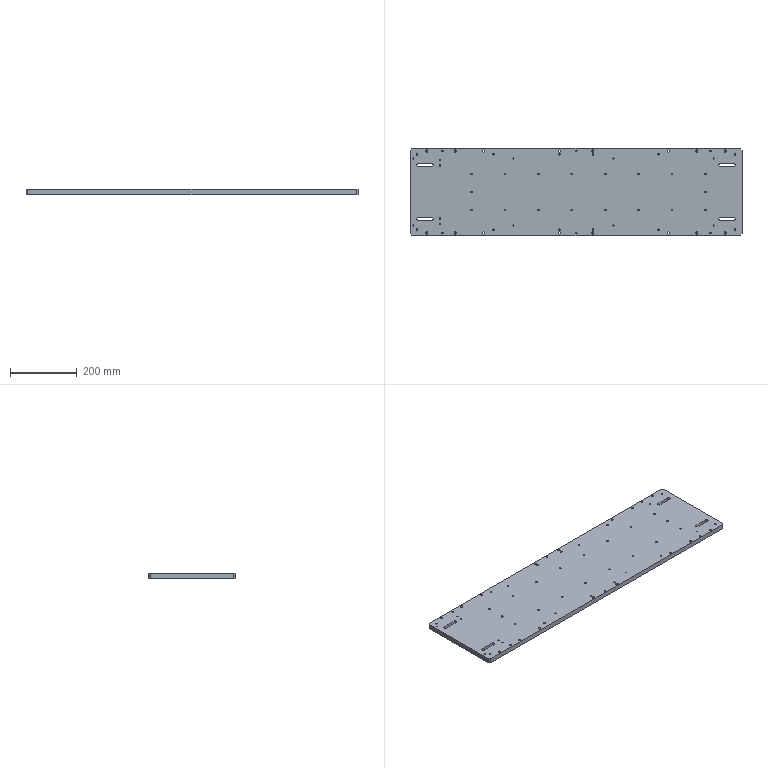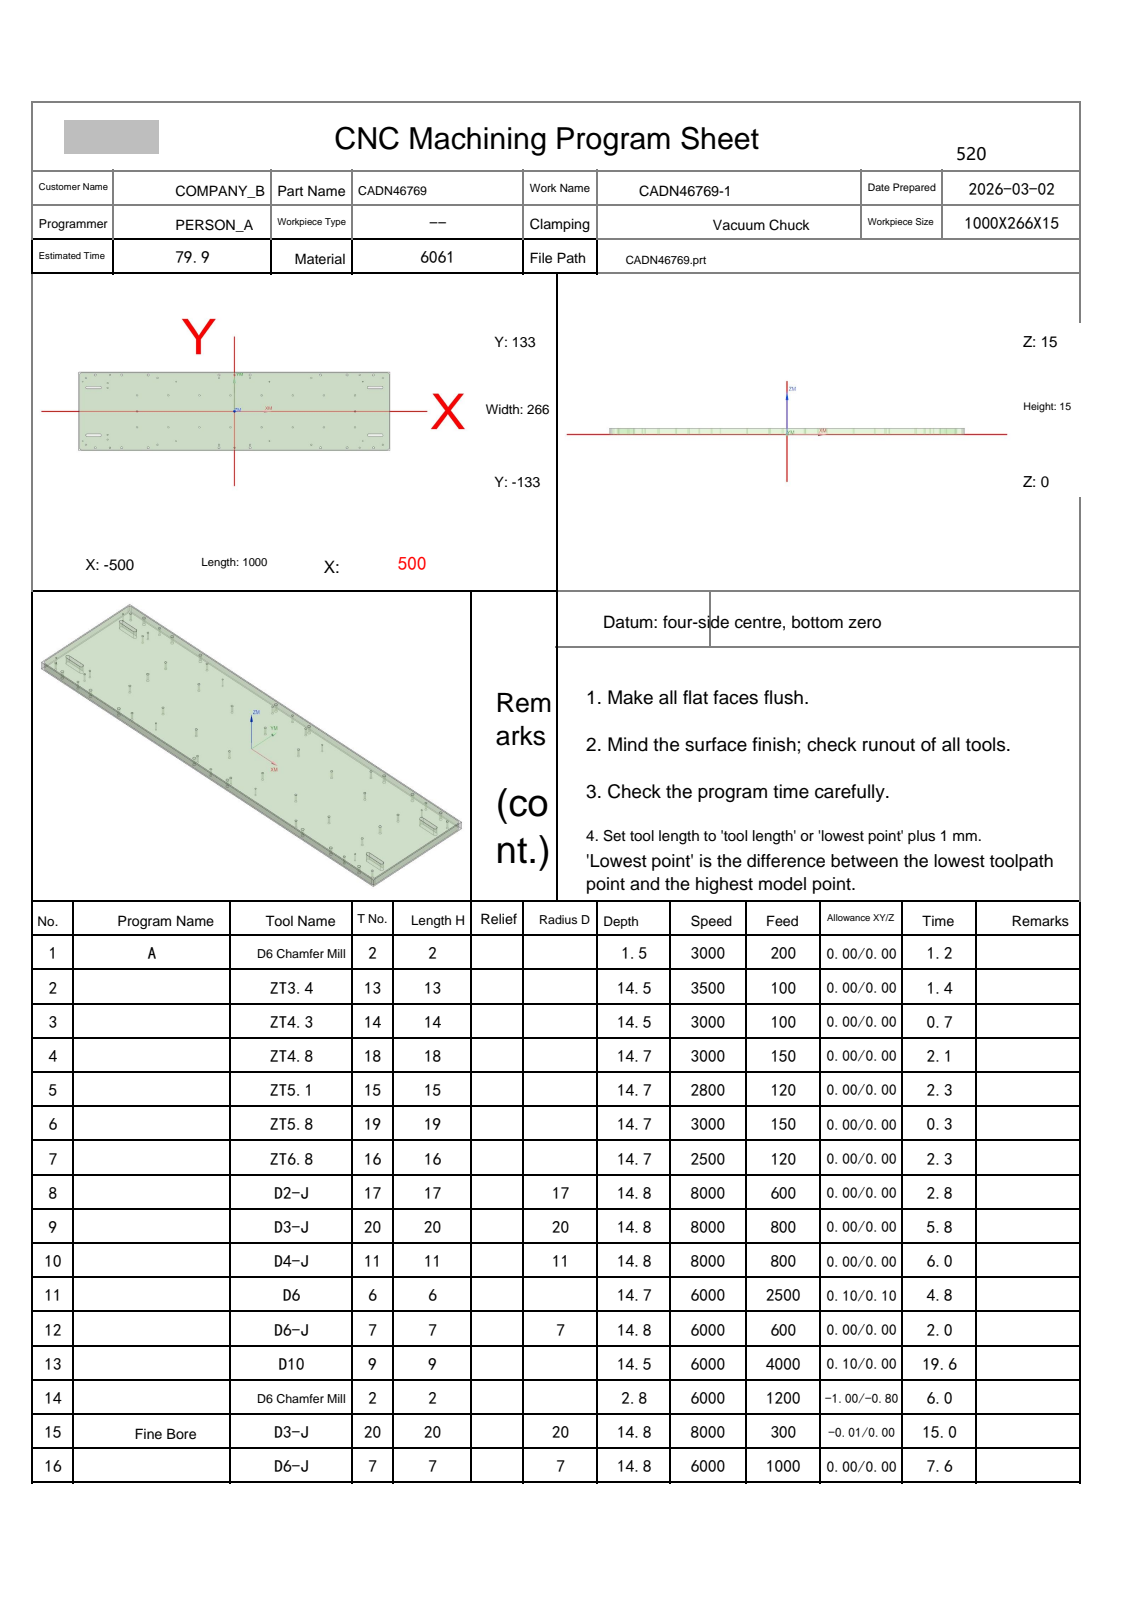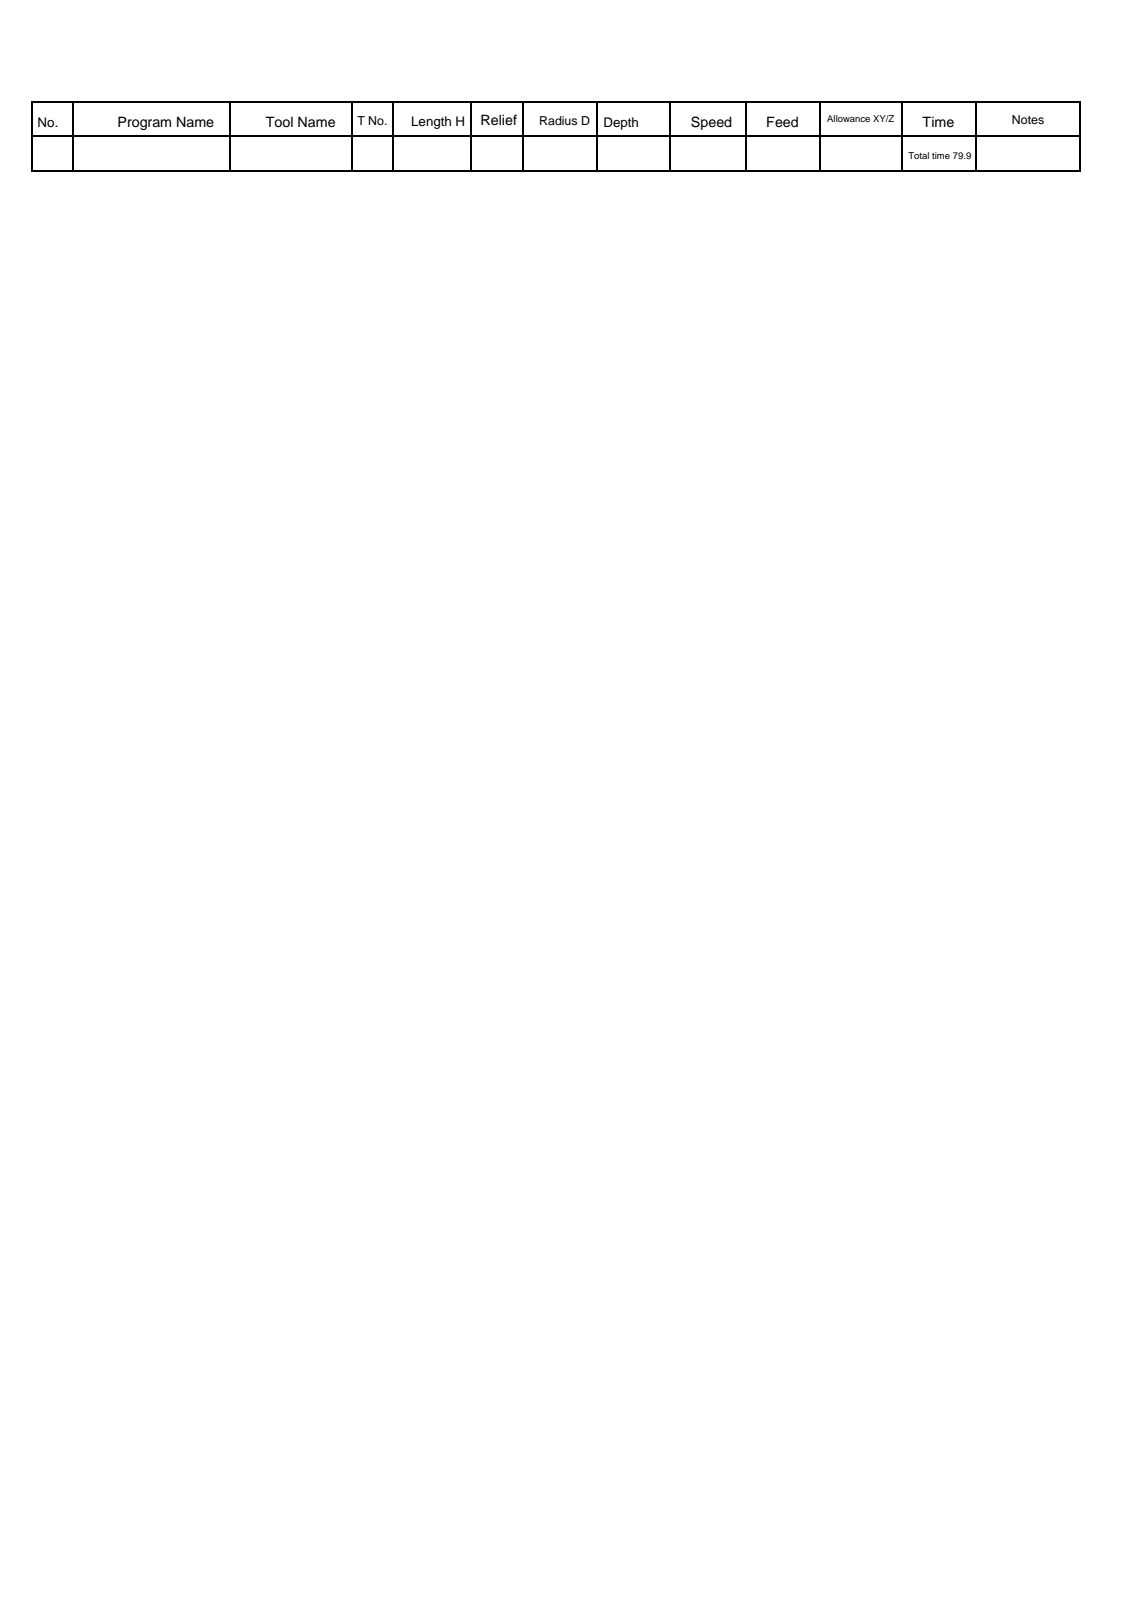NC program | NX | posted by the shop | part box 995 x 261 x 15 mm
Lines 5894 to 6746 of 14350:
N10 T11 M06
(D4-J  D=4. R=0. H=11 ce=0.00 di=0.00)
G00 G90 G54 X447.899 Y124.023 M03 S8000
G43 H11 Z45.
M08
Z15.5
G01 X447.739 Y124.154 Z15.489 F800.
X447.457 Y124.292 Z15.473
X447.152 Y124.362 Z15.456
X446.883 Y124.365 Z15.442
X446.571 Y124.301 Z15.425
X446.281 Y124.167 Z15.409
X446.031 Y123.969 Z15.392
X445.833 Y123.719 Z15.375
X445.699 Y123.429 Z15.359
X445.635 Y123.117 Z15.342
Y122.883 Z15.33
X445.699 Y122.571 Z15.313
X445.833 Y122.281 Z15.296
X446.031 Y122.031 Z15.28
X446.281 Y121.833 Z15.263
X446.571 Y121.699 Z15.246
X446.883 Y121.635 Z15.229
X447.117 Z15.217
X447.429 Y121.699 Z15.2
X447.719 Y121.833 Z15.184
X447.969 Y122.031 Z15.167
X448.167 Y122.281 Z15.15
X448.301 Y122.571 Z15.134
X448.365 Y122.883 Z15.117
Y123.117 Z15.105
X448.303 Y123.424 Z15.088
X448.173 Y123.708 Z15.072
X447.981 Y123.956 Z15.055
X447.739 Y124.154 Z15.039
X447.457 Y124.292 Z15.023
X447.152 Y124.362 Z15.006
X447.035 Y124.365 Z15.
G41 D11
X447. Y124.4
G03 X445.6 Y123. Z14.877 I0.0 J-1.4
X447. Y121.6 Z14.753 I1.4 J0.0
X448.4 Y123. Z14.63 I0.0 J1.4
X447. Y124.4 Z14.507 I-1.4 J0.0
X445.6 Y123. Z14.383 I0.0 J-1.4
X447. Y121.6 Z14.26 I1.4 J0.0
X448.4 Y123. Z14.137 I0.0 J1.4
X447. Y124.4 Z14.013 I-1.4 J0.0
X445.6 Y123. Z13.89 I0.0 J-1.4
X447. Y121.6 Z13.767 I1.4 J0.0
X448.4 Y123. Z13.643 I0.0 J1.4
X447. Y124.4 Z13.52 I-1.4 J0.0
X445.6 Y123. Z13.397 I0.0 J-1.4
X447. Y121.6 Z13.273 I1.4 J0.0
X448.4 Y123. Z13.15 I0.0 J1.4
X447. Y124.4 Z13.027 I-1.4 J0.0
X445.6 Y123. Z12.903 I0.0 J-1.4
X447. Y121.6 Z12.78 I1.4 J0.0
X448.4 Y123. Z12.657 I0.0 J1.4
X447. Y124.4 Z12.533 I-1.4 J0.0
X445.6 Y123. Z12.41 I0.0 J-1.4
X447. Y121.6 Z12.287 I1.4 J0.0
X448.4 Y123. Z12.163 I0.0 J1.4
X447. Y124.4 Z12.04 I-1.4 J0.0
X445.6 Y123. Z11.917 I0.0 J-1.4
X447. Y121.6 Z11.793 I1.4 J0.0
X448.4 Y123. Z11.67 I0.0 J1.4
X447. Y124.4 Z11.547 I-1.4 J0.0
X445.6 Y123. Z11.423 I0.0 J-1.4
X447. Y121.6 Z11.3 I1.4 J0.0
X448.4 Y123. Z11.177 I0.0 J1.4
X447. Y124.4 Z11.053 I-1.4 J0.0
X445.6 Y123. Z10.93 I0.0 J-1.4
X447. Y121.6 Z10.807 I1.4 J0.0
X448.4 Y123. Z10.683 I0.0 J1.4
X447. Y124.4 Z10.56 I-1.4 J0.0
X445.6 Y123. Z10.437 I0.0 J-1.4
X447. Y121.6 Z10.313 I1.4 J0.0
X448.4 Y123. Z10.19 I0.0 J1.4
X447. Y124.4 Z10.067 I-1.4 J0.0
X445.6 Y123. Z9.943 I0.0 J-1.4
X447. Y121.6 Z9.82 I1.4 J0.0
X448.4 Y123. Z9.697 I0.0 J1.4
X447. Y124.4 Z9.573 I-1.4 J0.0
X445.6 Y123. Z9.45 I0.0 J-1.4
X447. Y121.6 Z9.327 I1.4 J0.0
X448.4 Y123. Z9.203 I0.0 J1.4
X447. Y124.4 Z9.08 I-1.4 J0.0
X445.6 Y123. Z8.957 I0.0 J-1.4
X447. Y121.6 Z8.833 I1.4 J0.0
X448.4 Y123. Z8.71 I0.0 J1.4
X447. Y124.4 Z8.587 I-1.4 J0.0
X445.6 Y123. Z8.463 I0.0 J-1.4
X447. Y121.6 Z8.34 I1.4 J0.0
X448.4 Y123. Z8.217 I0.0 J1.4
X447. Y124.4 Z8.093 I-1.4 J0.0
X445.6 Y123. Z7.97 I0.0 J-1.4
X447. Y121.6 Z7.847 I1.4 J0.0
X448.4 Y123. Z7.723 I0.0 J1.4
X447. Y124.4 Z7.6 I-1.4 J0.0
X445.6 Y123. Z7.477 I0.0 J-1.4
X447. Y121.6 Z7.353 I1.4 J0.0
X448.4 Y123. Z7.23 I0.0 J1.4
X447. Y124.4 Z7.107 I-1.4 J0.0
X445.6 Y123. Z6.983 I0.0 J-1.4
X447. Y121.6 Z6.86 I1.4 J0.0
X448.4 Y123. Z6.737 I0.0 J1.4
X447. Y124.4 Z6.613 I-1.4 J0.0
X445.6 Y123. Z6.49 I0.0 J-1.4
X447. Y121.6 Z6.367 I1.4 J0.0
X448.4 Y123. Z6.243 I0.0 J1.4
X447. Y124.4 Z6.12 I-1.4 J0.0
X445.6 Y123. Z5.997 I0.0 J-1.4
X447. Y121.6 Z5.873 I1.4 J0.0
X448.4 Y123. Z5.75 I0.0 J1.4
X447. Y124.4 Z5.627 I-1.4 J0.0
X445.6 Y123. Z5.503 I0.0 J-1.4
X447. Y121.6 Z5.38 I1.4 J0.0
X448.4 Y123. Z5.257 I0.0 J1.4
X447. Y124.4 Z5.133 I-1.4 J0.0
X445.6 Y123. Z5.01 I0.0 J-1.4
X447. Y121.6 Z4.887 I1.4 J0.0
X448.4 Y123. Z4.763 I0.0 J1.4
X447. Y124.4 Z4.64 I-1.4 J0.0
X445.6 Y123. Z4.517 I0.0 J-1.4
X447. Y121.6 Z4.393 I1.4 J0.0
X448.4 Y123. Z4.27 I0.0 J1.4
X447. Y124.4 Z4.147 I-1.4 J0.0
X445.6 Y123. Z4.023 I0.0 J-1.4
X447. Y121.6 Z3.9 I1.4 J0.0
X448.4 Y123. Z3.777 I0.0 J1.4
X447. Y124.4 Z3.653 I-1.4 J0.0
X445.6 Y123. Z3.53 I0.0 J-1.4
X447. Y121.6 Z3.407 I1.4 J0.0
X448.4 Y123. Z3.283 I0.0 J1.4
X447. Y124.4 Z3.16 I-1.4 J0.0
X445.6 Y123. Z3.037 I0.0 J-1.4
X447. Y121.6 Z2.913 I1.4 J0.0
X448.4 Y123. Z2.79 I0.0 J1.4
X447. Y124.4 Z2.667 I-1.4 J0.0
X445.6 Y123. Z2.543 I0.0 J-1.4
X447. Y121.6 Z2.42 I1.4 J0.0
X448.4 Y123. Z2.297 I0.0 J1.4
X447. Y124.4 Z2.173 I-1.4 J0.0
X445.6 Y123. Z2.05 I0.0 J-1.4
X447. Y121.6 Z1.927 I1.4 J0.0
X448.4 Y123. Z1.803 I0.0 J1.4
X447. Y124.4 Z1.68 I-1.4 J0.0
X445.6 Y123. Z1.557 I0.0 J-1.4
X447. Y121.6 Z1.433 I1.4 J0.0
X448.4 Y123. Z1.31 I0.0 J1.4
X447. Y124.4 Z1.187 I-1.4 J0.0
X445.6 Y123. Z1.063 I0.0 J-1.4
X447. Y121.6 Z.94 I1.4 J0.0
X448.4 Y123. Z.817 I0.0 J1.4
X447. Y124.4 Z.693 I-1.4 J0.0
X445.6 Y123. Z.57 I0.0 J-1.4
X447. Y121.6 Z.447 I1.4 J0.0
X448.4 Y123. Z.323 I0.0 J1.4
X447. Y124.4 Z.2 I-1.4 J0.0
X445.6 Y123. I0.0 J-1.4
X447. Y121.6 I1.4 J0.0
X448.4 Y123. I0.0 J1.4
X447. Y124.4 I-1.4 J0.0
X446.605 Y124.343 I0.0 J-1.4
G01 X446.58 Y124.333
X446.566 Y124.308
X446.572 Y124.281
G40 X446.586 Y124.233
Z1.2
G00 Z45.
X362.899 Y124.023
Z15.5
G01 X362.739 Y124.154 Z15.489
X362.457 Y124.292 Z15.473
X362.152 Y124.362 Z15.456
X361.883 Y124.365 Z15.442
X361.571 Y124.301 Z15.425
X361.281 Y124.167 Z15.409
X361.031 Y123.969 Z15.392
X360.833 Y123.719 Z15.375
X360.699 Y123.429 Z15.359
X360.635 Y123.117 Z15.342
Y122.883 Z15.33
X360.699 Y122.571 Z15.313
X360.833 Y122.281 Z15.296
X361.031 Y122.031 Z15.28
X361.281 Y121.833 Z15.263
X361.571 Y121.699 Z15.246
X361.883 Y121.635 Z15.229
X362.117 Z15.217
X362.429 Y121.699 Z15.2
X362.719 Y121.833 Z15.184
X362.969 Y122.031 Z15.167
X363.167 Y122.281 Z15.15
X363.301 Y122.571 Z15.134
X363.365 Y122.883 Z15.117
Y123.117 Z15.105
X363.303 Y123.424 Z15.088
X363.173 Y123.708 Z15.072
X362.981 Y123.956 Z15.055
X362.739 Y124.154 Z15.039
X362.457 Y124.292 Z15.023
X362.152 Y124.362 Z15.006
X362.035 Y124.365 Z15.
G41 D11
X362. Y124.4
G03 X360.6 Y123. Z14.877 I0.0 J-1.4
X362. Y121.6 Z14.753 I1.4 J0.0
X363.4 Y123. Z14.63 I0.0 J1.4
X362. Y124.4 Z14.507 I-1.4 J0.0
X360.6 Y123. Z14.383 I0.0 J-1.4
X362. Y121.6 Z14.26 I1.4 J0.0
X363.4 Y123. Z14.137 I0.0 J1.4
X362. Y124.4 Z14.013 I-1.4 J0.0
X360.6 Y123. Z13.89 I0.0 J-1.4
X362. Y121.6 Z13.767 I1.4 J0.0
X363.4 Y123. Z13.643 I0.0 J1.4
X362. Y124.4 Z13.52 I-1.4 J0.0
X360.6 Y123. Z13.397 I0.0 J-1.4
X362. Y121.6 Z13.273 I1.4 J0.0
X363.4 Y123. Z13.15 I0.0 J1.4
X362. Y124.4 Z13.027 I-1.4 J0.0
X360.6 Y123. Z12.903 I0.0 J-1.4
X362. Y121.6 Z12.78 I1.4 J0.0
X363.4 Y123. Z12.657 I0.0 J1.4
X362. Y124.4 Z12.533 I-1.4 J0.0
X360.6 Y123. Z12.41 I0.0 J-1.4
X362. Y121.6 Z12.287 I1.4 J0.0
X363.4 Y123. Z12.163 I0.0 J1.4
X362. Y124.4 Z12.04 I-1.4 J0.0
X360.6 Y123. Z11.917 I0.0 J-1.4
X362. Y121.6 Z11.793 I1.4 J0.0
X363.4 Y123. Z11.67 I0.0 J1.4
X362. Y124.4 Z11.547 I-1.4 J0.0
X360.6 Y123. Z11.423 I0.0 J-1.4
X362. Y121.6 Z11.3 I1.4 J0.0
X363.4 Y123. Z11.177 I0.0 J1.4
X362. Y124.4 Z11.053 I-1.4 J0.0
X360.6 Y123. Z10.93 I0.0 J-1.4
X362. Y121.6 Z10.807 I1.4 J0.0
X363.4 Y123. Z10.683 I0.0 J1.4
X362. Y124.4 Z10.56 I-1.4 J0.0
X360.6 Y123. Z10.437 I0.0 J-1.4
X362. Y121.6 Z10.313 I1.4 J0.0
X363.4 Y123. Z10.19 I0.0 J1.4
X362. Y124.4 Z10.067 I-1.4 J0.0
X360.6 Y123. Z9.943 I0.0 J-1.4
X362. Y121.6 Z9.82 I1.4 J0.0
X363.4 Y123. Z9.697 I0.0 J1.4
X362. Y124.4 Z9.573 I-1.4 J0.0
X360.6 Y123. Z9.45 I0.0 J-1.4
X362. Y121.6 Z9.327 I1.4 J0.0
X363.4 Y123. Z9.203 I0.0 J1.4
X362. Y124.4 Z9.08 I-1.4 J0.0
X360.6 Y123. Z8.957 I0.0 J-1.4
X362. Y121.6 Z8.833 I1.4 J0.0
X363.4 Y123. Z8.71 I0.0 J1.4
X362. Y124.4 Z8.587 I-1.4 J0.0
X360.6 Y123. Z8.463 I0.0 J-1.4
X362. Y121.6 Z8.34 I1.4 J0.0
X363.4 Y123. Z8.217 I0.0 J1.4
X362. Y124.4 Z8.093 I-1.4 J0.0
X360.6 Y123. Z7.97 I0.0 J-1.4
X362. Y121.6 Z7.847 I1.4 J0.0
X363.4 Y123. Z7.723 I0.0 J1.4
X362. Y124.4 Z7.6 I-1.4 J0.0
X360.6 Y123. Z7.477 I0.0 J-1.4
X362. Y121.6 Z7.353 I1.4 J0.0
X363.4 Y123. Z7.23 I0.0 J1.4
X362. Y124.4 Z7.107 I-1.4 J0.0
X360.6 Y123. Z6.983 I0.0 J-1.4
X362. Y121.6 Z6.86 I1.4 J0.0
X363.4 Y123. Z6.737 I0.0 J1.4
X362. Y124.4 Z6.613 I-1.4 J0.0
X360.6 Y123. Z6.49 I0.0 J-1.4
X362. Y121.6 Z6.367 I1.4 J0.0
X363.4 Y123. Z6.243 I0.0 J1.4
X362. Y124.4 Z6.12 I-1.4 J0.0
X360.6 Y123. Z5.997 I0.0 J-1.4
X362. Y121.6 Z5.873 I1.4 J0.0
X363.4 Y123. Z5.75 I0.0 J1.4
X362. Y124.4 Z5.627 I-1.4 J0.0
X360.6 Y123. Z5.503 I0.0 J-1.4
X362. Y121.6 Z5.38 I1.4 J0.0
X363.4 Y123. Z5.257 I0.0 J1.4
X362. Y124.4 Z5.133 I-1.4 J0.0
X360.6 Y123. Z5.01 I0.0 J-1.4
X362. Y121.6 Z4.887 I1.4 J0.0
X363.4 Y123. Z4.763 I0.0 J1.4
X362. Y124.4 Z4.64 I-1.4 J0.0
X360.6 Y123. Z4.517 I0.0 J-1.4
X362. Y121.6 Z4.393 I1.4 J0.0
X363.4 Y123. Z4.27 I0.0 J1.4
X362. Y124.4 Z4.147 I-1.4 J0.0
X360.6 Y123. Z4.023 I0.0 J-1.4
X362. Y121.6 Z3.9 I1.4 J0.0
X363.4 Y123. Z3.777 I0.0 J1.4
X362. Y124.4 Z3.653 I-1.4 J0.0
X360.6 Y123. Z3.53 I0.0 J-1.4
X362. Y121.6 Z3.407 I1.4 J0.0
X363.4 Y123. Z3.283 I0.0 J1.4
X362. Y124.4 Z3.16 I-1.4 J0.0
X360.6 Y123. Z3.037 I0.0 J-1.4
X362. Y121.6 Z2.913 I1.4 J0.0
X363.4 Y123. Z2.79 I0.0 J1.4
X362. Y124.4 Z2.667 I-1.4 J0.0
X360.6 Y123. Z2.543 I0.0 J-1.4
X362. Y121.6 Z2.42 I1.4 J0.0
X363.4 Y123. Z2.297 I0.0 J1.4
X362. Y124.4 Z2.173 I-1.4 J0.0
X360.6 Y123. Z2.05 I0.0 J-1.4
X362. Y121.6 Z1.927 I1.4 J0.0
X363.4 Y123. Z1.803 I0.0 J1.4
X362. Y124.4 Z1.68 I-1.4 J0.0
X360.6 Y123. Z1.557 I0.0 J-1.4
X362. Y121.6 Z1.433 I1.4 J0.0
X363.4 Y123. Z1.31 I0.0 J1.4
X362. Y124.4 Z1.187 I-1.4 J0.0
X360.6 Y123. Z1.063 I0.0 J-1.4
X362. Y121.6 Z.94 I1.4 J0.0
X363.4 Y123. Z.817 I0.0 J1.4
X362. Y124.4 Z.693 I-1.4 J0.0
X360.6 Y123. Z.57 I0.0 J-1.4
X362. Y121.6 Z.447 I1.4 J0.0
X363.4 Y123. Z.323 I0.0 J1.4
X362. Y124.4 Z.2 I-1.4 J0.0
X360.6 Y123. I0.0 J-1.4
X362. Y121.6 I1.4 J0.0
X363.4 Y123. I0.0 J1.4
X362. Y124.4 I-1.4 J0.0
X361.605 Y124.343 I0.0 J-1.4
G01 X361.58 Y124.333
X361.566 Y124.308
X361.572 Y124.281
G40 X361.586 Y124.233
Z1.2
G00 Z45.
X277.899 Y124.023
Z15.5
G01 X277.739 Y124.154 Z15.489
X277.457 Y124.292 Z15.473
X277.152 Y124.362 Z15.456
X276.883 Y124.365 Z15.442
X276.571 Y124.301 Z15.425
X276.281 Y124.167 Z15.409
X276.031 Y123.969 Z15.392
X275.833 Y123.719 Z15.375
X275.699 Y123.429 Z15.359
X275.635 Y123.117 Z15.342
Y122.883 Z15.33
X275.699 Y122.571 Z15.313
X275.833 Y122.281 Z15.296
X276.031 Y122.031 Z15.28
X276.281 Y121.833 Z15.263
X276.571 Y121.699 Z15.246
X276.883 Y121.635 Z15.229
X277.117 Z15.217
X277.429 Y121.699 Z15.2
X277.719 Y121.833 Z15.184
X277.969 Y122.031 Z15.167
X278.167 Y122.281 Z15.15
X278.301 Y122.571 Z15.134
X278.365 Y122.883 Z15.117
Y123.117 Z15.105
X278.303 Y123.424 Z15.088
X278.173 Y123.708 Z15.072
X277.981 Y123.956 Z15.055
X277.739 Y124.154 Z15.039
X277.457 Y124.292 Z15.023
X277.152 Y124.362 Z15.006
X277.035 Y124.365 Z15.
G41 D11
X277. Y124.4
G03 X275.6 Y123. Z14.877 I0.0 J-1.4
X277. Y121.6 Z14.753 I1.4 J0.0
X278.4 Y123. Z14.63 I0.0 J1.4
X277. Y124.4 Z14.507 I-1.4 J0.0
X275.6 Y123. Z14.383 I0.0 J-1.4
X277. Y121.6 Z14.26 I1.4 J0.0
X278.4 Y123. Z14.137 I0.0 J1.4
X277. Y124.4 Z14.013 I-1.4 J0.0
X275.6 Y123. Z13.89 I0.0 J-1.4
X277. Y121.6 Z13.767 I1.4 J0.0
X278.4 Y123. Z13.643 I0.0 J1.4
X277. Y124.4 Z13.52 I-1.4 J0.0
X275.6 Y123. Z13.397 I0.0 J-1.4
X277. Y121.6 Z13.273 I1.4 J0.0
X278.4 Y123. Z13.15 I0.0 J1.4
X277. Y124.4 Z13.027 I-1.4 J0.0
X275.6 Y123. Z12.903 I0.0 J-1.4
X277. Y121.6 Z12.78 I1.4 J0.0
X278.4 Y123. Z12.657 I0.0 J1.4
X277. Y124.4 Z12.533 I-1.4 J0.0
X275.6 Y123. Z12.41 I0.0 J-1.4
X277. Y121.6 Z12.287 I1.4 J0.0
X278.4 Y123. Z12.163 I0.0 J1.4
X277. Y124.4 Z12.04 I-1.4 J0.0
X275.6 Y123. Z11.917 I0.0 J-1.4
X277. Y121.6 Z11.793 I1.4 J0.0
X278.4 Y123. Z11.67 I0.0 J1.4
X277. Y124.4 Z11.547 I-1.4 J0.0
X275.6 Y123. Z11.423 I0.0 J-1.4
X277. Y121.6 Z11.3 I1.4 J0.0
X278.4 Y123. Z11.177 I0.0 J1.4
X277. Y124.4 Z11.053 I-1.4 J0.0
X275.6 Y123. Z10.93 I0.0 J-1.4
X277. Y121.6 Z10.807 I1.4 J0.0
X278.4 Y123. Z10.683 I0.0 J1.4
X277. Y124.4 Z10.56 I-1.4 J0.0
X275.6 Y123. Z10.437 I0.0 J-1.4
X277. Y121.6 Z10.313 I1.4 J0.0
X278.4 Y123. Z10.19 I0.0 J1.4
X277. Y124.4 Z10.067 I-1.4 J0.0
X275.6 Y123. Z9.943 I0.0 J-1.4
X277. Y121.6 Z9.82 I1.4 J0.0
X278.4 Y123. Z9.697 I0.0 J1.4
X277. Y124.4 Z9.573 I-1.4 J0.0
X275.6 Y123. Z9.45 I0.0 J-1.4
X277. Y121.6 Z9.327 I1.4 J0.0
X278.4 Y123. Z9.203 I0.0 J1.4
X277. Y124.4 Z9.08 I-1.4 J0.0
X275.6 Y123. Z8.957 I0.0 J-1.4
X277. Y121.6 Z8.833 I1.4 J0.0
X278.4 Y123. Z8.71 I0.0 J1.4
X277. Y124.4 Z8.587 I-1.4 J0.0
X275.6 Y123. Z8.463 I0.0 J-1.4
X277. Y121.6 Z8.34 I1.4 J0.0
X278.4 Y123. Z8.217 I0.0 J1.4
X277. Y124.4 Z8.093 I-1.4 J0.0
X275.6 Y123. Z7.97 I0.0 J-1.4
X277. Y121.6 Z7.847 I1.4 J0.0
X278.4 Y123. Z7.723 I0.0 J1.4
X277. Y124.4 Z7.6 I-1.4 J0.0
X275.6 Y123. Z7.477 I0.0 J-1.4
X277. Y121.6 Z7.353 I1.4 J0.0
X278.4 Y123. Z7.23 I0.0 J1.4
X277. Y124.4 Z7.107 I-1.4 J0.0
X275.6 Y123. Z6.983 I0.0 J-1.4
X277. Y121.6 Z6.86 I1.4 J0.0
X278.4 Y123. Z6.737 I0.0 J1.4
X277. Y124.4 Z6.613 I-1.4 J0.0
X275.6 Y123. Z6.49 I0.0 J-1.4
X277. Y121.6 Z6.367 I1.4 J0.0
X278.4 Y123. Z6.243 I0.0 J1.4
X277. Y124.4 Z6.12 I-1.4 J0.0
X275.6 Y123. Z5.997 I0.0 J-1.4
X277. Y121.6 Z5.873 I1.4 J0.0
X278.4 Y123. Z5.75 I0.0 J1.4
X277. Y124.4 Z5.627 I-1.4 J0.0
X275.6 Y123. Z5.503 I0.0 J-1.4
X277. Y121.6 Z5.38 I1.4 J0.0
X278.4 Y123. Z5.257 I0.0 J1.4
X277. Y124.4 Z5.133 I-1.4 J0.0
X275.6 Y123. Z5.01 I0.0 J-1.4
X277. Y121.6 Z4.887 I1.4 J0.0
X278.4 Y123. Z4.763 I0.0 J1.4
X277. Y124.4 Z4.64 I-1.4 J0.0
X275.6 Y123. Z4.517 I0.0 J-1.4
X277. Y121.6 Z4.393 I1.4 J0.0
X278.4 Y123. Z4.27 I0.0 J1.4
X277. Y124.4 Z4.147 I-1.4 J0.0
X275.6 Y123. Z4.023 I0.0 J-1.4
X277. Y121.6 Z3.9 I1.4 J0.0
X278.4 Y123. Z3.777 I0.0 J1.4
X277. Y124.4 Z3.653 I-1.4 J0.0
X275.6 Y123. Z3.53 I0.0 J-1.4
X277. Y121.6 Z3.407 I1.4 J0.0
X278.4 Y123. Z3.283 I0.0 J1.4
X277. Y124.4 Z3.16 I-1.4 J0.0
X275.6 Y123. Z3.037 I0.0 J-1.4
X277. Y121.6 Z2.913 I1.4 J0.0
X278.4 Y123. Z2.79 I0.0 J1.4
X277. Y124.4 Z2.667 I-1.4 J0.0
X275.6 Y123. Z2.543 I0.0 J-1.4
X277. Y121.6 Z2.42 I1.4 J0.0
X278.4 Y123. Z2.297 I0.0 J1.4
X277. Y124.4 Z2.173 I-1.4 J0.0
X275.6 Y123. Z2.05 I0.0 J-1.4
X277. Y121.6 Z1.927 I1.4 J0.0
X278.4 Y123. Z1.803 I0.0 J1.4
X277. Y124.4 Z1.68 I-1.4 J0.0
X275.6 Y123. Z1.557 I0.0 J-1.4
X277. Y121.6 Z1.433 I1.4 J0.0
X278.4 Y123. Z1.31 I0.0 J1.4
X277. Y124.4 Z1.187 I-1.4 J0.0
X275.6 Y123. Z1.063 I0.0 J-1.4
X277. Y121.6 Z.94 I1.4 J0.0
X278.4 Y123. Z.817 I0.0 J1.4
X277. Y124.4 Z.693 I-1.4 J0.0
X275.6 Y123. Z.57 I0.0 J-1.4
X277. Y121.6 Z.447 I1.4 J0.0
X278.4 Y123. Z.323 I0.0 J1.4
X277. Y124.4 Z.2 I-1.4 J0.0
X275.6 Y123. I0.0 J-1.4
X277. Y121.6 I1.4 J0.0
X278.4 Y123. I0.0 J1.4
X277. Y124.4 I-1.4 J0.0
X276.605 Y124.343 I0.0 J-1.4
G01 X276.58 Y124.333
X276.566 Y124.308
X276.572 Y124.281
G40 X276.586 Y124.233
Z1.2
G00 Z45.
X51.399 Y124.023
Z15.5
G01 X51.239 Y124.154 Z15.489
X50.957 Y124.292 Z15.473
X50.652 Y124.362 Z15.456
X50.383 Y124.365 Z15.442
X50.071 Y124.301 Z15.425
X49.781 Y124.167 Z15.409
X49.531 Y123.969 Z15.392
X49.333 Y123.719 Z15.375
X49.199 Y123.429 Z15.359
X49.135 Y123.117 Z15.342
Y122.883 Z15.33
X49.199 Y122.571 Z15.313
X49.333 Y122.281 Z15.296
X49.531 Y122.031 Z15.28
X49.781 Y121.833 Z15.263
X50.071 Y121.699 Z15.246
X50.383 Y121.635 Z15.229
X50.617 Z15.217
X50.929 Y121.699 Z15.2
X51.219 Y121.833 Z15.184
X51.469 Y122.031 Z15.167
X51.667 Y122.281 Z15.15
X51.801 Y122.571 Z15.134
X51.865 Y122.883 Z15.117
Y123.117 Z15.105
X51.803 Y123.424 Z15.088
X51.673 Y123.708 Z15.072
X51.481 Y123.956 Z15.055
X51.239 Y124.154 Z15.039
X50.957 Y124.292 Z15.023
X50.652 Y124.362 Z15.006
X50.535 Y124.365 Z15.
G41 D11
X50.5 Y124.4
G03 X49.1 Y123. Z14.877 I0.0 J-1.4
X50.5 Y121.6 Z14.753 I1.4 J0.0
X51.9 Y123. Z14.63 I0.0 J1.4
X50.5 Y124.4 Z14.507 I-1.4 J0.0
X49.1 Y123. Z14.383 I0.0 J-1.4
X50.5 Y121.6 Z14.26 I1.4 J0.0
X51.9 Y123. Z14.137 I0.0 J1.4
X50.5 Y124.4 Z14.013 I-1.4 J0.0
X49.1 Y123. Z13.89 I0.0 J-1.4
X50.5 Y121.6 Z13.767 I1.4 J0.0
X51.9 Y123. Z13.643 I0.0 J1.4
X50.5 Y124.4 Z13.52 I-1.4 J0.0
X49.1 Y123. Z13.397 I0.0 J-1.4
X50.5 Y121.6 Z13.273 I1.4 J0.0
X51.9 Y123. Z13.15 I0.0 J1.4
X50.5 Y124.4 Z13.027 I-1.4 J0.0
X49.1 Y123. Z12.903 I0.0 J-1.4
X50.5 Y121.6 Z12.78 I1.4 J0.0
X51.9 Y123. Z12.657 I0.0 J1.4
X50.5 Y124.4 Z12.533 I-1.4 J0.0
X49.1 Y123. Z12.41 I0.0 J-1.4
X50.5 Y121.6 Z12.287 I1.4 J0.0
X51.9 Y123. Z12.163 I0.0 J1.4
X50.5 Y124.4 Z12.04 I-1.4 J0.0
X49.1 Y123. Z11.917 I0.0 J-1.4
X50.5 Y121.6 Z11.793 I1.4 J0.0
X51.9 Y123. Z11.67 I0.0 J1.4
X50.5 Y124.4 Z11.547 I-1.4 J0.0
X49.1 Y123. Z11.423 I0.0 J-1.4
X50.5 Y121.6 Z11.3 I1.4 J0.0
X51.9 Y123. Z11.177 I0.0 J1.4
X50.5 Y124.4 Z11.053 I-1.4 J0.0
X49.1 Y123. Z10.93 I0.0 J-1.4
X50.5 Y121.6 Z10.807 I1.4 J0.0
X51.9 Y123. Z10.683 I0.0 J1.4
X50.5 Y124.4 Z10.56 I-1.4 J0.0
X49.1 Y123. Z10.437 I0.0 J-1.4
X50.5 Y121.6 Z10.313 I1.4 J0.0
X51.9 Y123. Z10.19 I0.0 J1.4
X50.5 Y124.4 Z10.067 I-1.4 J0.0
X49.1 Y123. Z9.943 I0.0 J-1.4
X50.5 Y121.6 Z9.82 I1.4 J0.0
X51.9 Y123. Z9.697 I0.0 J1.4
X50.5 Y124.4 Z9.573 I-1.4 J0.0
X49.1 Y123. Z9.45 I0.0 J-1.4
X50.5 Y121.6 Z9.327 I1.4 J0.0
X51.9 Y123. Z9.203 I0.0 J1.4
X50.5 Y124.4 Z9.08 I-1.4 J0.0
X49.1 Y123. Z8.957 I0.0 J-1.4
X50.5 Y121.6 Z8.833 I1.4 J0.0
X51.9 Y123. Z8.71 I0.0 J1.4
X50.5 Y124.4 Z8.587 I-1.4 J0.0
X49.1 Y123. Z8.463 I0.0 J-1.4
X50.5 Y121.6 Z8.34 I1.4 J0.0
X51.9 Y123. Z8.217 I0.0 J1.4
X50.5 Y124.4 Z8.093 I-1.4 J0.0
X49.1 Y123. Z7.97 I0.0 J-1.4
X50.5 Y121.6 Z7.847 I1.4 J0.0
X51.9 Y123. Z7.723 I0.0 J1.4
X50.5 Y124.4 Z7.6 I-1.4 J0.0
X49.1 Y123. Z7.477 I0.0 J-1.4
X50.5 Y121.6 Z7.353 I1.4 J0.0
X51.9 Y123. Z7.23 I0.0 J1.4
X50.5 Y124.4 Z7.107 I-1.4 J0.0
X49.1 Y123. Z6.983 I0.0 J-1.4
X50.5 Y121.6 Z6.86 I1.4 J0.0
X51.9 Y123. Z6.737 I0.0 J1.4
X50.5 Y124.4 Z6.613 I-1.4 J0.0
X49.1 Y123. Z6.49 I0.0 J-1.4
X50.5 Y121.6 Z6.367 I1.4 J0.0
X51.9 Y123. Z6.243 I0.0 J1.4
X50.5 Y124.4 Z6.12 I-1.4 J0.0
X49.1 Y123. Z5.997 I0.0 J-1.4
X50.5 Y121.6 Z5.873 I1.4 J0.0
X51.9 Y123. Z5.75 I0.0 J1.4
X50.5 Y124.4 Z5.627 I-1.4 J0.0
X49.1 Y123. Z5.503 I0.0 J-1.4
X50.5 Y121.6 Z5.38 I1.4 J0.0
X51.9 Y123. Z5.257 I0.0 J1.4
X50.5 Y124.4 Z5.133 I-1.4 J0.0
X49.1 Y123. Z5.01 I0.0 J-1.4
X50.5 Y121.6 Z4.887 I1.4 J0.0
X51.9 Y123. Z4.763 I0.0 J1.4
X50.5 Y124.4 Z4.64 I-1.4 J0.0
X49.1 Y123. Z4.517 I0.0 J-1.4
X50.5 Y121.6 Z4.393 I1.4 J0.0
X51.9 Y123. Z4.27 I0.0 J1.4
X50.5 Y124.4 Z4.147 I-1.4 J0.0
X49.1 Y123. Z4.023 I0.0 J-1.4
X50.5 Y121.6 Z3.9 I1.4 J0.0
X51.9 Y123. Z3.777 I0.0 J1.4
X50.5 Y124.4 Z3.653 I-1.4 J0.0
X49.1 Y123. Z3.53 I0.0 J-1.4
X50.5 Y121.6 Z3.407 I1.4 J0.0
X51.9 Y123. Z3.283 I0.0 J1.4
X50.5 Y124.4 Z3.16 I-1.4 J0.0
X49.1 Y123. Z3.037 I0.0 J-1.4
X50.5 Y121.6 Z2.913 I1.4 J0.0
X51.9 Y123. Z2.79 I0.0 J1.4
X50.5 Y124.4 Z2.667 I-1.4 J0.0
X49.1 Y123. Z2.543 I0.0 J-1.4
X50.5 Y121.6 Z2.42 I1.4 J0.0
X51.9 Y123. Z2.297 I0.0 J1.4
X50.5 Y124.4 Z2.173 I-1.4 J0.0
X49.1 Y123. Z2.05 I0.0 J-1.4
X50.5 Y121.6 Z1.927 I1.4 J0.0
X51.9 Y123. Z1.803 I0.0 J1.4
X50.5 Y124.4 Z1.68 I-1.4 J0.0
X49.1 Y123. Z1.557 I0.0 J-1.4
X50.5 Y121.6 Z1.433 I1.4 J0.0
X51.9 Y123. Z1.31 I0.0 J1.4
X50.5 Y124.4 Z1.187 I-1.4 J0.0
X49.1 Y123. Z1.063 I0.0 J-1.4
X50.5 Y121.6 Z.94 I1.4 J0.0
X51.9 Y123. Z.817 I0.0 J1.4
X50.5 Y124.4 Z.693 I-1.4 J0.0
X49.1 Y123. Z.57 I0.0 J-1.4
X50.5 Y121.6 Z.447 I1.4 J0.0
X51.9 Y123. Z.323 I0.0 J1.4
X50.5 Y124.4 Z.2 I-1.4 J0.0
X49.1 Y123. I0.0 J-1.4
X50.5 Y121.6 I1.4 J0.0
X51.9 Y123. I0.0 J1.4
X50.5 Y124.4 I-1.4 J0.0
X50.105 Y124.343 I0.0 J-1.4
G01 X50.08 Y124.333
X50.066 Y124.308
X50.072 Y124.281
G40 X50.086 Y124.233
Z1.2
G00 Z45.
X-48.601 Y124.023
Z15.5
G01 X-48.761 Y124.154 Z15.489
X-49.043 Y124.292 Z15.473
X-49.348 Y124.362 Z15.456
X-49.617 Y124.365 Z15.442
X-49.929 Y124.301 Z15.425
X-50.219 Y124.167 Z15.409
X-50.469 Y123.969 Z15.392
X-50.667 Y123.719 Z15.375
X-50.801 Y123.429 Z15.359
X-50.865 Y123.117 Z15.342
Y122.883 Z15.33
X-50.801 Y122.571 Z15.313
X-50.667 Y122.281 Z15.296
X-50.469 Y122.031 Z15.28
X-50.219 Y121.833 Z15.263
X-49.929 Y121.699 Z15.246
X-49.617 Y121.635 Z15.229
X-49.383 Z15.217
X-49.071 Y121.699 Z15.2
X-48.781 Y121.833 Z15.184
X-48.531 Y122.031 Z15.167
X-48.333 Y122.281 Z15.15
X-48.199 Y122.571 Z15.134
X-48.135 Y122.883 Z15.117
Y123.117 Z15.105
X-48.197 Y123.424 Z15.088
X-48.327 Y123.708 Z15.072
X-48.519 Y123.956 Z15.055
X-48.761 Y124.154 Z15.039
X-49.043 Y124.292 Z15.023
X-49.348 Y124.362 Z15.006
X-49.465 Y124.365 Z15.
G41 D11
X-49.5 Y124.4
G03 X-50.9 Y123. Z14.877 I0.0 J-1.4
X-49.5 Y121.6 Z14.753 I1.4 J0.0
X-48.1 Y123. Z14.63 I0.0 J1.4
X-49.5 Y124.4 Z14.507 I-1.4 J0.0
X-50.9 Y123. Z14.383 I0.0 J-1.4
X-49.5 Y121.6 Z14.26 I1.4 J0.0
X-48.1 Y123. Z14.137 I0.0 J1.4
X-49.5 Y124.4 Z14.013 I-1.4 J0.0
X-50.9 Y123. Z13.89 I0.0 J-1.4
X-49.5 Y121.6 Z13.767 I1.4 J0.0
X-48.1 Y123. Z13.643 I0.0 J1.4
X-49.5 Y124.4 Z13.52 I-1.4 J0.0
X-50.9 Y123. Z13.397 I0.0 J-1.4
X-49.5 Y121.6 Z13.273 I1.4 J0.0
X-48.1 Y123. Z13.15 I0.0 J1.4
X-49.5 Y124.4 Z13.027 I-1.4 J0.0
X-50.9 Y123. Z12.903 I0.0 J-1.4
X-49.5 Y121.6 Z12.78 I1.4 J0.0
X-48.1 Y123. Z12.657 I0.0 J1.4
X-49.5 Y124.4 Z12.533 I-1.4 J0.0
X-50.9 Y123. Z12.41 I0.0 J-1.4
X-49.5 Y121.6 Z12.287 I1.4 J0.0
X-48.1 Y123. Z12.163 I0.0 J1.4
X-49.5 Y124.4 Z12.04 I-1.4 J0.0
X-50.9 Y123. Z11.917 I0.0 J-1.4
X-49.5 Y121.6 Z11.793 I1.4 J0.0
X-48.1 Y123. Z11.67 I0.0 J1.4
X-49.5 Y124.4 Z11.547 I-1.4 J0.0
X-50.9 Y123. Z11.423 I0.0 J-1.4
X-49.5 Y121.6 Z11.3 I1.4 J0.0
X-48.1 Y123. Z11.177 I0.0 J1.4
X-49.5 Y124.4 Z11.053 I-1.4 J0.0
X-50.9 Y123. Z10.93 I0.0 J-1.4
X-49.5 Y121.6 Z10.807 I1.4 J0.0
X-48.1 Y123. Z10.683 I0.0 J1.4
X-49.5 Y124.4 Z10.56 I-1.4 J0.0
X-50.9 Y123. Z10.437 I0.0 J-1.4
X-49.5 Y121.6 Z10.313 I1.4 J0.0
X-48.1 Y123. Z10.19 I0.0 J1.4
X-49.5 Y124.4 Z10.067 I-1.4 J0.0
X-50.9 Y123. Z9.943 I0.0 J-1.4
X-49.5 Y121.6 Z9.82 I1.4 J0.0
X-48.1 Y123. Z9.697 I0.0 J1.4
X-49.5 Y124.4 Z9.573 I-1.4 J0.0
X-50.9 Y123. Z9.45 I0.0 J-1.4
X-49.5 Y121.6 Z9.327 I1.4 J0.0
X-48.1 Y123. Z9.203 I0.0 J1.4
X-49.5 Y124.4 Z9.08 I-1.4 J0.0
X-50.9 Y123. Z8.957 I0.0 J-1.4
X-49.5 Y121.6 Z8.833 I1.4 J0.0
X-48.1 Y123. Z8.71 I0.0 J1.4
X-49.5 Y124.4 Z8.587 I-1.4 J0.0
X-50.9 Y123. Z8.463 I0.0 J-1.4
X-49.5 Y121.6 Z8.34 I1.4 J0.0
X-48.1 Y123. Z8.217 I0.0 J1.4
X-49.5 Y124.4 Z8.093 I-1.4 J0.0
X-50.9 Y123. Z7.97 I0.0 J-1.4
X-49.5 Y121.6 Z7.847 I1.4 J0.0
X-48.1 Y123. Z7.723 I0.0 J1.4
X-49.5 Y124.4 Z7.6 I-1.4 J0.0
X-50.9 Y123. Z7.477 I0.0 J-1.4
X-49.5 Y121.6 Z7.353 I1.4 J0.0
X-48.1 Y123. Z7.23 I0.0 J1.4
X-49.5 Y124.4 Z7.107 I-1.4 J0.0
X-50.9 Y123. Z6.983 I0.0 J-1.4
X-49.5 Y121.6 Z6.86 I1.4 J0.0
X-48.1 Y123. Z6.737 I0.0 J1.4
X-49.5 Y124.4 Z6.613 I-1.4 J0.0
X-50.9 Y123. Z6.49 I0.0 J-1.4
X-49.5 Y121.6 Z6.367 I1.4 J0.0
X-48.1 Y123. Z6.243 I0.0 J1.4
X-49.5 Y124.4 Z6.12 I-1.4 J0.0
X-50.9 Y123. Z5.997 I0.0 J-1.4
X-49.5 Y121.6 Z5.873 I1.4 J0.0
X-48.1 Y123. Z5.75 I0.0 J1.4
X-49.5 Y124.4 Z5.627 I-1.4 J0.0
X-50.9 Y123. Z5.503 I0.0 J-1.4
X-49.5 Y121.6 Z5.38 I1.4 J0.0
X-48.1 Y123. Z5.257 I0.0 J1.4
X-49.5 Y124.4 Z5.133 I-1.4 J0.0
X-50.9 Y123. Z5.01 I0.0 J-1.4
X-49.5 Y121.6 Z4.887 I1.4 J0.0
X-48.1 Y123. Z4.763 I0.0 J1.4
X-49.5 Y124.4 Z4.64 I-1.4 J0.0
X-50.9 Y123. Z4.517 I0.0 J-1.4
X-49.5 Y121.6 Z4.393 I1.4 J0.0
X-48.1 Y123. Z4.27 I0.0 J1.4
X-49.5 Y124.4 Z4.147 I-1.4 J0.0
X-50.9 Y123. Z4.023 I0.0 J-1.4
X-49.5 Y121.6 Z3.9 I1.4 J0.0
X-48.1 Y123. Z3.777 I0.0 J1.4
X-49.5 Y124.4 Z3.653 I-1.4 J0.0
X-50.9 Y123. Z3.53 I0.0 J-1.4
X-49.5 Y121.6 Z3.407 I1.4 J0.0
X-48.1 Y123. Z3.283 I0.0 J1.4
X-49.5 Y124.4 Z3.16 I-1.4 J0.0
X-50.9 Y123. Z3.037 I0.0 J-1.4
X-49.5 Y121.6 Z2.913 I1.4 J0.0
X-48.1 Y123. Z2.79 I0.0 J1.4
X-49.5 Y124.4 Z2.667 I-1.4 J0.0
X-50.9 Y123. Z2.543 I0.0 J-1.4
X-49.5 Y121.6 Z2.42 I1.4 J0.0
X-48.1 Y123. Z2.297 I0.0 J1.4
X-49.5 Y124.4 Z2.173 I-1.4 J0.0
X-50.9 Y123. Z2.05 I0.0 J-1.4
X-49.5 Y121.6 Z1.927 I1.4 J0.0
X-48.1 Y123. Z1.803 I0.0 J1.4
X-49.5 Y124.4 Z1.68 I-1.4 J0.0
X-50.9 Y123. Z1.557 I0.0 J-1.4
X-49.5 Y121.6 Z1.433 I1.4 J0.0
X-48.1 Y123. Z1.31 I0.0 J1.4
X-49.5 Y124.4 Z1.187 I-1.4 J0.0
X-50.9 Y123. Z1.063 I0.0 J-1.4
X-49.5 Y121.6 Z.94 I1.4 J0.0
X-48.1 Y123. Z.817 I0.0 J1.4
X-49.5 Y124.4 Z.693 I-1.4 J0.0
X-50.9 Y123. Z.57 I0.0 J-1.4
X-49.5 Y121.6 Z.447 I1.4 J0.0
X-48.1 Y123. Z.323 I0.0 J1.4
X-49.5 Y124.4 Z.2 I-1.4 J0.0
X-50.9 Y123. I0.0 J-1.4
X-49.5 Y121.6 I1.4 J0.0
X-48.1 Y123. I0.0 J1.4
X-49.5 Y124.4 I-1.4 J0.0
X-49.895 Y124.343 I0.0 J-1.4
G01 X-49.92 Y124.333
X-49.934 Y124.308
X-49.928 Y124.281
G40 X-49.914 Y124.233
Z1.2
G00 Z45.
X-276.101 Y124.023
Z15.5
G01 X-276.261 Y124.154 Z15.489
X-276.543 Y124.292 Z15.473
X-276.848 Y124.362 Z15.456
X-277.117 Y124.365 Z15.442
X-277.429 Y124.301 Z15.425
X-277.719 Y124.167 Z15.409
X-277.969 Y123.969 Z15.392
X-278.167 Y123.719 Z15.375
X-278.301 Y123.429 Z15.359
X-278.365 Y123.117 Z15.342
Y122.883 Z15.33
X-278.301 Y122.571 Z15.313